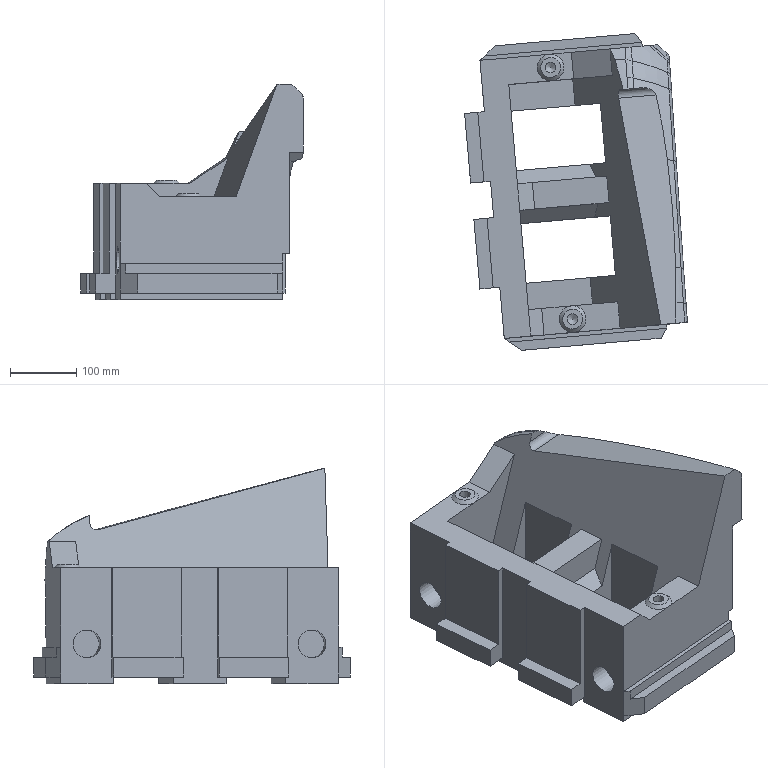Part | NX | features solid 2 | 1 solid | 183 faces | box 335.358 x 476.552 x 324.297 mm | volume 15944108 mm3 | spline 88 | plane 82 | cylinder 9 | cone 4 | commonest cylinder face diameters 20 x3 16 x2 42 x2 40 x1 80 x1